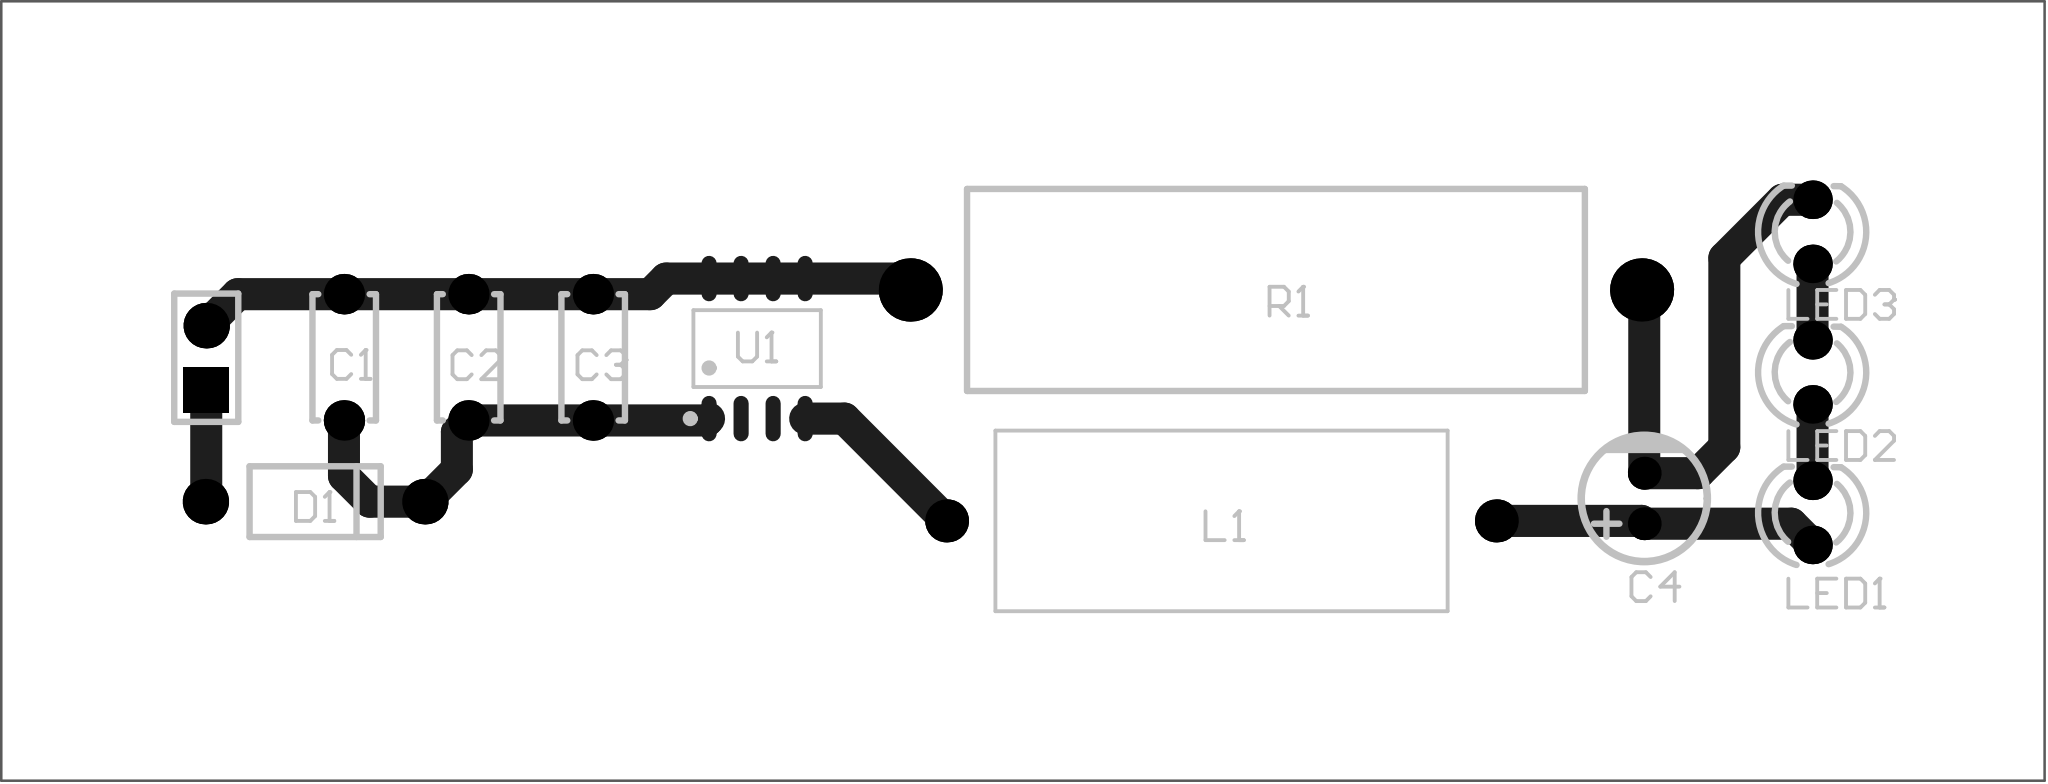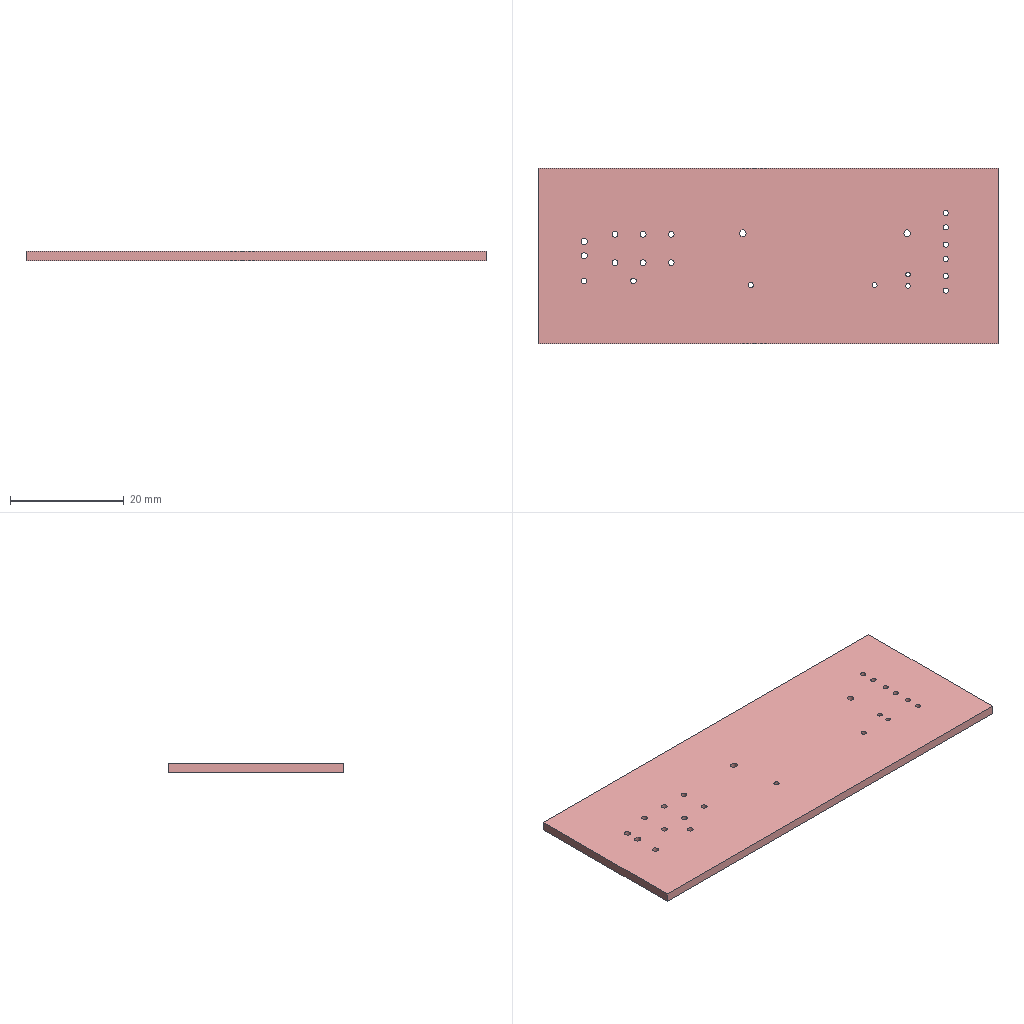Circuit board layout | Altium Designer | box 81 x 30.9 x 1.6 mm
Layer stack:
# Altium Designer layer stack of  (unit mm; dielectric type: 0 none, 1 core, 2 prepreg, 3 surface material)
index,name,kind,layer,copper_thickness_mm,dielectric_type,dielectric_thickness_mm,dielectric_material,dielectric_constant
0,Top Paste Mask Layer,other,,,,,,
1,Top Silkscreen Layer,other,,,,,,
2,Top Solder Mask Layer,dielectric,,,3,0.01,,3.3
3,Top Layer,copper,Top Layer,0.035,,,,
4,Dielectric1,dielectric,,,3,1.51,FR4,4.5
5,Bottom Layer,copper,Bottom Layer,0.035,,,,
6,Bottom Solder Mask Layer,dielectric,,,3,0.01,,3.3
7,Bottom Silkscreen Layer,other,,,,,,
8,Bottom Paste Mask Layer,other,,,,,,
# drill layer pairs: low layer,high layer
drill_pair,Top Layer,Bottom Layer
Part placement:
Designator,Comment,Layer,Footprint,Center-X(mm),Center-Y(mm),Rotation
C1,100nF,TopLayer,CAP-TH_L5.0-W2.5-P5.00-D1.0,83.439,86.614,90
C2,100nF,TopLayer,CAP-TH_L5.0-W2.5-P5.00-D1.0,88.375,86.614,90
C3,10nF,TopLayer,CAP-TH_L5.0-W2.5-P5.00-D1.0,93.311,86.614,90
C4,10uF,TopLayer,CAP-TH_BD5.0-P2.00-D0.8-FD-10UF50VC110GL,135.001,81.026,90
D1,,TopLayer,DO_1N4007,82.296,80.899,180
H1,,TopLayer,HDR-TH_2P-P2.54-V-M-1,77.978,86.598,90
LED1,,TopLayer,LED_TH-3mm,141.674,80.456,90
LED2,,TopLayer,LED_TH-3mm,141.674,86.019,90
LED3,,TopLayer,LED_TH-3mm,141.674,91.583,90
R1,0.68Ω,TopLayer,Res_5W,120.396,89.281,0
U1,PT4501C,TopLayer,SOP-8_L4.9-W3.9-P1.27-LS6.0-BL-EP,99.822,86.96,0
L1,47uH,TopLayer,IND-TH_BD7.0-L17.8-P21.80-D0.8,118.237,80.137,0
Pad and via stacks:
# Altium Designer via and pad stacks of  (unit mm). Each distinct definition once, with the count of objects using it.
# via: kind,start_layer,end_layer,hole_mm,diameter_mm,mode(0 simple;1 top-mid-bottom;2 full stack),diameter_per_layer,count,example_net
# pad: kind,layer,hole_mm,hole_type(0 round;1 square;2 slot),plating,top_size,top_shape(1 round;2 rect;3 octagon;9 rounded rect),mid_size,bottom_size,mode,footprint,size_per_layer,count,example
pad,Multi-Layer,1,0,plated,1.6x1.6,1,1.6x1.6,1.6x1.6,0,CAP-TH_L5.0-W2.5-P5.00-D1.0,,6,C1.1
pad,Multi-Layer,0.8,0,plated,1.3x1.3,1,1.3x1.3,1.3x1.3,0,CAP-TH_BD5.0-P2.00-D0.8-FD-10UF50VC110GL,,2,C4.1
pad,Multi-Layer,1,0,plated,1.8x1.8,1,1.8x1.8,1.8x1.8,0,DO_1N4007,,2,D1.1
pad,Multi-Layer,1.1,0,plated,1.8x1.8,1,1.8x1.8,1.8x1.8,0,HDR-TH_2P-P2.54-V-M-1,,1,H1.2
pad,Multi-Layer,1.1,0,plated,1.8x1.8,2,1.8x1.8,1.8x1.8,0,HDR-TH_2P-P2.54-V-M-1,,1,H1.1
pad,Multi-Layer,0.9144,0,plated,1.524x1.524,1,1.524x1.524,1.524x1.524,0,LED_TH-3mm,,6,LED1.1
pad,Multi-Layer,1.2,0,plated,2.5x2.5,1,2.5x2.5,2.5x2.5,0,Res_5W,,2,R1.1
pad,Multi-Layer,0.9,0,plated,1.7x1.7,1,1.7x1.7,1.7x1.7,0,IND-TH_BD7.0-L17.8-P21.80-D0.8,,2,L1.2
pad,Top Layer,0,0,plated,0.6x1.8,1,0.6x1.8,0.6x1.8,0,SOP-8_L4.9-W3.9-P1.27-LS6.0-BL-EP,,8,U1.1